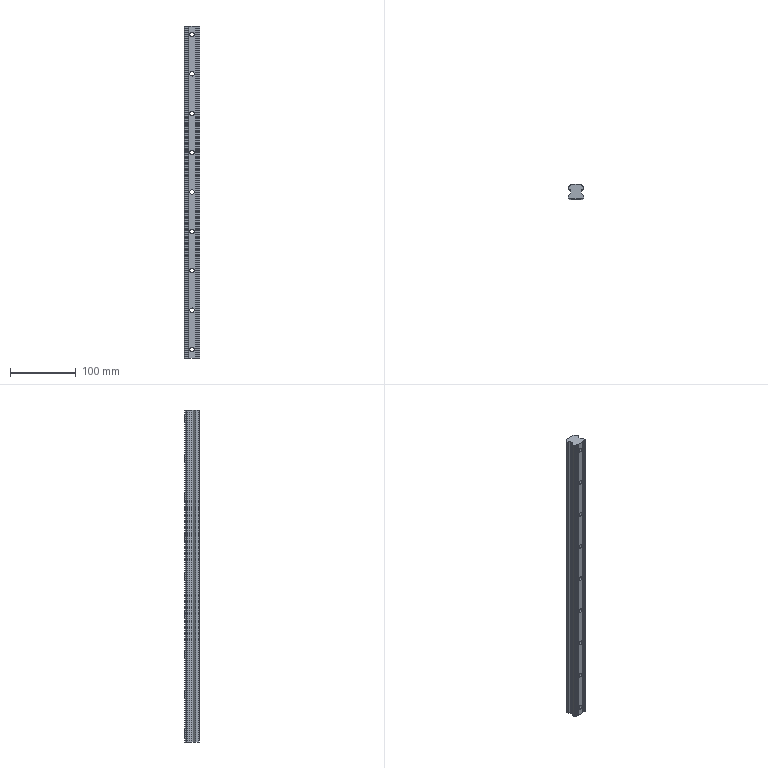Part | STEP file | HGH25 rail | 1 solid | 79 faces | box 23 x 22 x 506 mm | volume 212116 mm3 | cylinder 40 | plane 39 | commonest cylinder face diameters 11 x18 6.6 x16 4.6 x4 7 x2